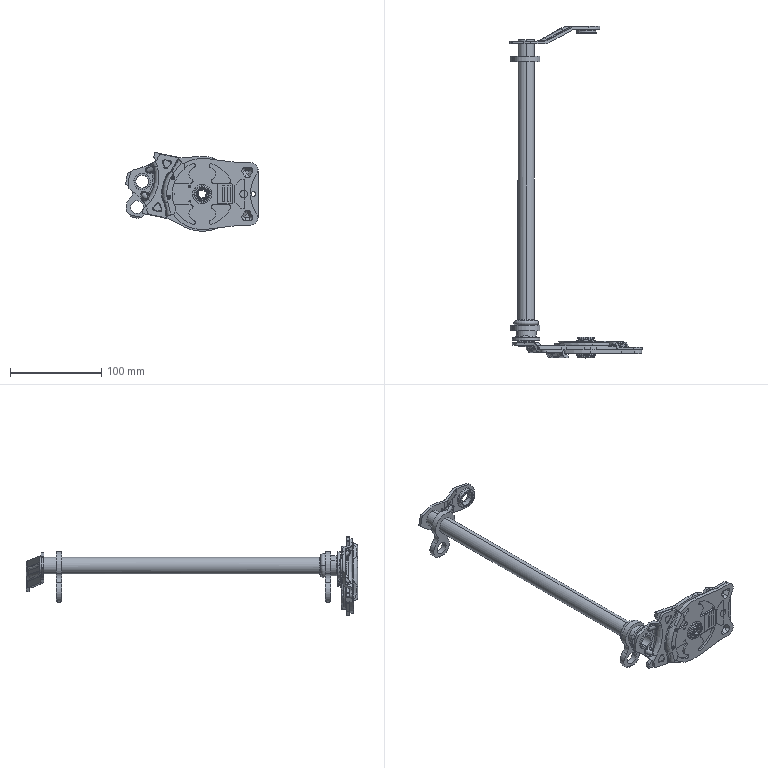Part | NX | features BREP 22 | 24 solids | 2440 faces | box 145.049 x 363 x 86.299 mm | volume 158665 mm3 | cylinder 924 | plane 661 | spline 436 | torus 219 | cone 168 | sphere 32 | commonest cylinder face diameters 0.3 x169 0.6 x144 1 x58 4 x40 2 x38 3 x32